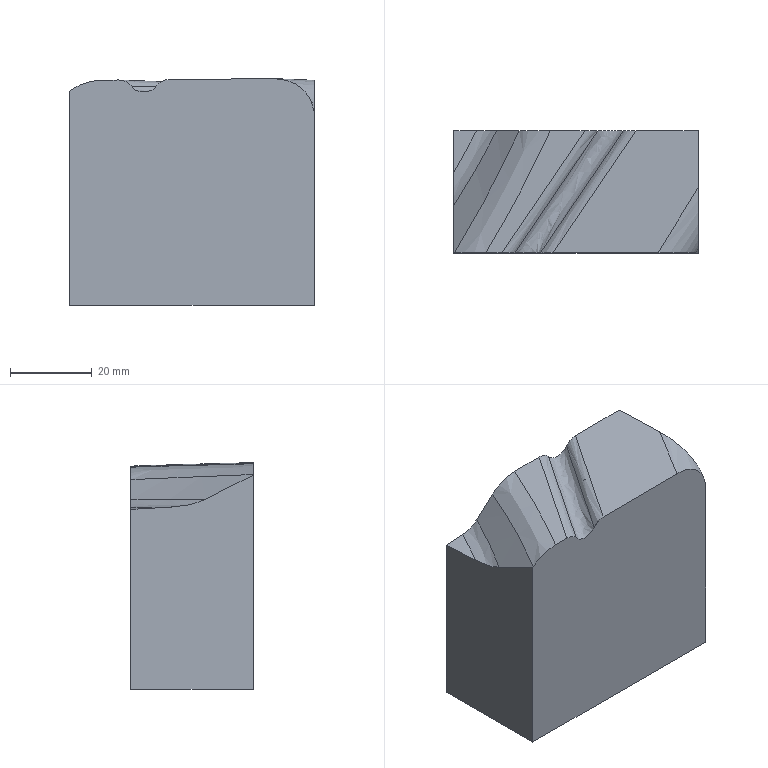Part | NX | features solid 2 | 1 solid | 17 faces | box 60 x 30 x 55.649 mm | volume 96446 mm3 | spline 12 | plane 5
STEP:
#1=CARTESIAN_POINT('',(484.173,-140.,-5.));
#2=VERTEX_POINT('',#1);
#3=CARTESIAN_POINT('',(424.173,-140.,-5.));
#4=VERTEX_POINT('',#3);
#5=CARTESIAN_POINT('',(484.173,-140.,-5.));
#6=DIRECTION('',(1.,0.,0.));
#7=VECTOR('',#6,1000.);
#8=LINE('',#5,#7);
#9=EDGE_CURVE('',#2,#4,#8,.F.);
#10=ORIENTED_EDGE('',*,*,#9,.F.);
#11=CARTESIAN_POINT('',(484.173,-170.,-5.));
#12=VERTEX_POINT('',#11);
#13=CARTESIAN_POINT('',(484.173,-140.,-5.));
#14=DIRECTION('',(0.,1.,0.));
#15=VECTOR('',#14,1000.);
#16=LINE('',#13,#15);
#17=EDGE_CURVE('',#2,#12,#16,.F.);
#18=ORIENTED_EDGE('',*,*,#17,.T.);
#19=CARTESIAN_POINT('',(424.173,-170.,-5.));
#20=VERTEX_POINT('',#19);
#21=CARTESIAN_POINT('',(374.173,-170.,-5.));
#22=DIRECTION('',(-1.,0.,0.));
#23=VECTOR('',#22,1000.);
#24=LINE('',#21,#23);
#25=EDGE_CURVE('',#12,#20,#24,.T.);
#26=ORIENTED_EDGE('',*,*,#25,.T.);
#27=CARTESIAN_POINT('',(424.173,-140.,-5.));
#28=DIRECTION('',(0.,1.,0.));
#29=VECTOR('',#28,1000.);
#30=LINE('',#27,#29);
#31=EDGE_CURVE('',#4,#20,#30,.F.);
#32=ORIENTED_EDGE('',*,*,#31,.F.);
#33=EDGE_LOOP('',(#10,#18,#26,#32));
#34=FACE_BOUND('',#33,.T.);
#35=CARTESIAN_POINT('',(374.173,-140.,-5.));
#36=DIRECTION('',(0.,0.,-1.));
#37=DIRECTION('',(-1.,0.,0.));
#38=AXIS2_PLACEMENT_3D('',#35,#36,#37);
#39=PLANE('',#38);
#40=ADVANCED_FACE('',(#34),#39,.T.);
#41=CARTESIAN_POINT('',(424.173,-170.,47.58));
#42=VERTEX_POINT('',#41);
#43=CARTESIAN_POINT('',(424.173,-170.,115.));
#44=DIRECTION('',(0.,0.,1.));
#45=VECTOR('',#44,1000.);
#46=LINE('',#43,#45);
#47=EDGE_CURVE('',#42,#20,#46,.F.);
#48=ORIENTED_EDGE('',*,*,#47,.T.);
#49=ORIENTED_EDGE('',*,*,#25,.F.);
#50=CARTESIAN_POINT('',(484.173,-170.,42.661));
#51=VERTEX_POINT('',#50);
#52=CARTESIAN_POINT('',(484.173,-170.,115.));
#53=DIRECTION('',(0.,0.,-1.));
#54=VECTOR('',#53,1000.);
#55=LINE('',#52,#54);
#56=EDGE_CURVE('',#51,#12,#55,.T.);
#57=ORIENTED_EDGE('',*,*,#56,.F.);
#58=CARTESIAN_POINT('',(483.509,-170.,44.696));
#59=VERTEX_POINT('',#58);
#60=CARTESIAN_POINT('',(483.509,-170.,44.695));
#61=CARTESIAN_POINT('',(483.73,-170.,44.017));
#62=CARTESIAN_POINT('',(483.952,-170.,43.339));
#63=CARTESIAN_POINT('',(484.173,-170.,42.661));
#64=B_SPLINE_CURVE_WITH_KNOTS('',3,(#60,#61,#62,#63),.UNSPECIFIED.,.F.,.F.,(4,4),(0.017,0.01914),.UNSPECIFIED.);
#65=EDGE_CURVE('',#59,#51,#64,.T.);
#66=ORIENTED_EDGE('',*,*,#65,.F.);
#67=CARTESIAN_POINT('',(474.524,-170.,50.648));
#68=VERTEX_POINT('',#67);
#69=CARTESIAN_POINT('',(474.524,-170.,50.648));
#70=CARTESIAN_POINT('',(476.454,-170.,50.62));
#71=CARTESIAN_POINT('',(480.234,-170.,49.577));
#72=CARTESIAN_POINT('',(482.907,-170.,46.539));
#73=CARTESIAN_POINT('',(483.508,-170.,44.696));
#74=B_SPLINE_CURVE_WITH_KNOTS('',3,(#69,#70,#71,#72,#73),.UNSPECIFIED.,.F.,.F.,(4,1,4),(0.,0.005687,0.01137),.UNSPECIFIED.);
#75=EDGE_CURVE('',#68,#59,#74,.T.);
#76=ORIENTED_EDGE('',*,*,#75,.F.);
#77=CARTESIAN_POINT('',(474.268,-170.,50.649));
#78=VERTEX_POINT('',#77);
#79=CARTESIAN_POINT('',(474.268,-170.,50.649));
#80=CARTESIAN_POINT('',(474.354,-170.,50.649));
#81=CARTESIAN_POINT('',(474.439,-170.,50.649));
#82=CARTESIAN_POINT('',(474.524,-170.,50.648));
#83=B_SPLINE_CURVE_WITH_KNOTS('',3,(#79,#80,#81,#82),.UNSPECIFIED.,.F.,.F.,(4,4),(0.,0.0002558),.UNSPECIFIED.);
#84=EDGE_CURVE('',#78,#68,#83,.T.);
#85=ORIENTED_EDGE('',*,*,#84,.F.);
#86=CARTESIAN_POINT('',(448.584,-170.,50.424));
#87=VERTEX_POINT('',#86);
#88=CARTESIAN_POINT('',(484.734,-170.,50.74));
#89=DIRECTION('',(-1.,0.,-0.008731));
#90=VECTOR('',#89,1000.);
#91=LINE('',#88,#90);
#92=EDGE_CURVE('',#87,#78,#91,.F.);
#93=ORIENTED_EDGE('',*,*,#92,.F.);
#94=CARTESIAN_POINT('',(445.49,-170.,48.897));
#95=VERTEX_POINT('',#94);
#96=CARTESIAN_POINT('',(445.49,-170.,48.897));
#97=CARTESIAN_POINT('',(446.157,-170.,49.903));
#98=CARTESIAN_POINT('',(447.38,-170.,50.414));
#99=CARTESIAN_POINT('',(448.584,-170.,50.424));
#100=B_SPLINE_CURVE_WITH_KNOTS('',3,(#96,#97,#98,#99),.UNSPECIFIED.,.F.,.F.,(4,4),(0.0000186,0.003585),.UNSPECIFIED.);
#101=EDGE_CURVE('',#95,#87,#100,.T.);
#102=ORIENTED_EDGE('',*,*,#101,.F.);
#103=CARTESIAN_POINT('',(439.21,-170.,48.842));
#104=VERTEX_POINT('',#103);
#105=CARTESIAN_POINT('',(439.21,-170.,48.842));
#106=CARTESIAN_POINT('',(440.629,-170.,46.903));
#107=CARTESIAN_POINT('',(444.144,-170.,46.868));
#108=CARTESIAN_POINT('',(445.49,-170.,48.896));
#109=B_SPLINE_CURVE_WITH_KNOTS('',3,(#105,#106,#107,#108),.UNSPECIFIED.,.F.,.F.,(4,4),(0.0007156,0.007904),.UNSPECIFIED.);
#110=EDGE_CURVE('',#104,#95,#109,.T.);
#111=ORIENTED_EDGE('',*,*,#110,.F.);
#112=CARTESIAN_POINT('',(436.025,-170.,50.315));
#113=VERTEX_POINT('',#112);
#114=CARTESIAN_POINT('',(436.025,-170.,50.315));
#115=CARTESIAN_POINT('',(437.248,-170.,50.325));
#116=CARTESIAN_POINT('',(438.485,-170.,49.832));
#117=CARTESIAN_POINT('',(439.21,-170.,48.842));
#118=B_SPLINE_CURVE_WITH_KNOTS('',3,(#114,#115,#116,#117),.UNSPECIFIED.,.F.,.F.,(4,4),(0.00002144,0.003637),.UNSPECIFIED.);
#119=EDGE_CURVE('',#113,#104,#118,.T.);
#120=ORIENTED_EDGE('',*,*,#119,.F.);
#121=CARTESIAN_POINT('',(432.047,-170.,50.28));
#122=VERTEX_POINT('',#121);
#123=CARTESIAN_POINT('',(484.734,-170.,50.74));
#124=DIRECTION('',(-1.,0.,-0.008731));
#125=VECTOR('',#124,1000.);
#126=LINE('',#123,#125);
#127=EDGE_CURVE('',#122,#113,#126,.F.);
#128=ORIENTED_EDGE('',*,*,#127,.F.);
#129=CARTESIAN_POINT('',(424.373,-170.,47.733));
#130=VERTEX_POINT('',#129);
#131=CARTESIAN_POINT('',(424.373,-170.,47.733));
#132=CARTESIAN_POINT('',(426.555,-170.,49.407));
#133=CARTESIAN_POINT('',(429.292,-170.,50.256));
#134=CARTESIAN_POINT('',(432.047,-170.,50.28));
#135=B_SPLINE_CURVE_WITH_KNOTS('',3,(#131,#132,#133,#134),.UNSPECIFIED.,.F.,.F.,(4,4),(-0.0009759,0.007265),.UNSPECIFIED.);
#136=EDGE_CURVE('',#130,#122,#135,.T.);
#137=ORIENTED_EDGE('',*,*,#136,.F.);
#138=CARTESIAN_POINT('',(424.173,-170.,47.58));
#139=CARTESIAN_POINT('',(424.24,-170.,47.631));
#140=CARTESIAN_POINT('',(424.306,-170.,47.682));
#141=CARTESIAN_POINT('',(424.373,-170.,47.733));
#142=B_SPLINE_CURVE_WITH_KNOTS('',3,(#138,#139,#140,#141),.UNSPECIFIED.,.F.,.F.,(4,4),(0.,0.0002516),.UNSPECIFIED.);
#143=EDGE_CURVE('',#42,#130,#142,.T.);
#144=ORIENTED_EDGE('',*,*,#143,.F.);
#145=EDGE_LOOP('',(#48,#49,#57,#66,#76,#85,#93,#102,#111,#120,#128,#137,#144));
#146=FACE_BOUND('',#145,.T.);
#147=CARTESIAN_POINT('',(484.173,-170.,115.));
#148=DIRECTION('',(0.,-1.,0.));
#149=DIRECTION('',(0.,0.,-1.));
#150=AXIS2_PLACEMENT_3D('',#147,#148,#149);
#151=PLANE('',#150);
#152=ADVANCED_FACE('',(#146),#151,.T.);
#153=CARTESIAN_POINT('',(434.724,-140.,41.512));
#154=VERTEX_POINT('',#153);
#155=CARTESIAN_POINT('',(429.796,-140.,39.524));
#156=VERTEX_POINT('',#155);
#157=CARTESIAN_POINT('',(434.724,-140.,41.512));
#158=CARTESIAN_POINT('',(433.368,-140.,40.305));
#159=CARTESIAN_POINT('',(431.606,-140.,39.634));
#160=CARTESIAN_POINT('',(429.796,-140.,39.524));
#161=B_SPLINE_CURVE_WITH_KNOTS('',3,(#157,#158,#159,#160),.UNSPECIFIED.,.F.,.F.,(4,4),(0.,0.005426),.UNSPECIFIED.);
#162=EDGE_CURVE('',#154,#156,#161,.T.);
#163=ORIENTED_EDGE('',*,*,#162,.F.);
#164=CARTESIAN_POINT('',(440.182,-140.,46.484));
#165=VERTEX_POINT('',#164);
#166=CARTESIAN_POINT('',(440.182,-140.,46.484));
#167=CARTESIAN_POINT('',(438.381,-140.,44.806));
#168=CARTESIAN_POINT('',(436.562,-140.,43.148));
#169=CARTESIAN_POINT('',(434.724,-140.,41.512));
#170=B_SPLINE_CURVE_WITH_KNOTS('',3,(#166,#167,#168,#169),.UNSPECIFIED.,.F.,.F.,(4,4),(0.003756,0.01114),.UNSPECIFIED.);
#171=EDGE_CURVE('',#165,#154,#170,.T.);
#172=ORIENTED_EDGE('',*,*,#171,.F.);
#173=CARTESIAN_POINT('',(447.906,-140.,49.476));
#174=VERTEX_POINT('',#173);
#175=CARTESIAN_POINT('',(447.906,-140.,49.476));
#176=CARTESIAN_POINT('',(445.063,-140.,49.451));
#177=CARTESIAN_POINT('',(442.263,-140.,48.423));
#178=CARTESIAN_POINT('',(440.182,-140.,46.484));
#179=B_SPLINE_CURVE_WITH_KNOTS('',3,(#175,#176,#177,#178),.UNSPECIFIED.,.F.,.F.,(4,4),(0.,0.0084),.UNSPECIFIED.);
#180=EDGE_CURVE('',#174,#165,#179,.T.);
#181=ORIENTED_EDGE('',*,*,#180,.F.);
#182=CARTESIAN_POINT('',(456.404,-140.,49.55));
#183=VERTEX_POINT('',#182);
#184=CARTESIAN_POINT('',(484.742,-140.,49.797));
#185=DIRECTION('',(-1.,0.,-0.008731));
#186=VECTOR('',#185,1000.);
#187=LINE('',#184,#186);
#188=EDGE_CURVE('',#183,#174,#187,.T.);
#189=ORIENTED_EDGE('',*,*,#188,.F.);
#190=CARTESIAN_POINT('',(459.589,-140.,48.077));
#191=VERTEX_POINT('',#190);
#192=CARTESIAN_POINT('',(459.589,-140.,48.077));
#193=CARTESIAN_POINT('',(458.865,-140.,49.066));
#194=CARTESIAN_POINT('',(457.625,-140.,49.561));
#195=CARTESIAN_POINT('',(456.404,-140.,49.55));
#196=B_SPLINE_CURVE_WITH_KNOTS('',3,(#192,#193,#194,#195),.UNSPECIFIED.,.F.,.F.,(4,4),(0.00001889,0.00364),.UNSPECIFIED.);
#197=EDGE_CURVE('',#191,#183,#196,.T.);
#198=ORIENTED_EDGE('',*,*,#197,.F.);
#199=CARTESIAN_POINT('',(465.869,-140.,48.132));
#200=VERTEX_POINT('',#199);
#201=CARTESIAN_POINT('',(465.869,-140.,48.132));
#202=CARTESIAN_POINT('',(465.195,-140.,47.116));
#203=CARTESIAN_POINT('',(462.737,-140.,46.1));
#204=CARTESIAN_POINT('',(460.304,-140.,47.1));
#205=CARTESIAN_POINT('',(459.589,-140.,48.077));
#206=B_SPLINE_CURVE_WITH_KNOTS('',3,(#201,#202,#203,#204,#205),.UNSPECIFIED.,.F.,.F.,(4,1,4),(0.,0.003598,0.007195),.UNSPECIFIED.);
#207=EDGE_CURVE('',#200,#191,#206,.T.);
#208=ORIENTED_EDGE('',*,*,#207,.F.);
#209=CARTESIAN_POINT('',(468.963,-140.,49.66));
#210=VERTEX_POINT('',#209);
#211=CARTESIAN_POINT('',(468.963,-140.,49.66));
#212=CARTESIAN_POINT('',(467.759,-140.,49.649));
#213=CARTESIAN_POINT('',(466.537,-140.,49.139));
#214=CARTESIAN_POINT('',(465.868,-140.,48.132));
#215=B_SPLINE_CURVE_WITH_KNOTS('',3,(#211,#212,#213,#214),.UNSPECIFIED.,.F.,.F.,(4,4),(0.00002143,0.003581),.UNSPECIFIED.);
#216=EDGE_CURVE('',#210,#200,#215,.T.);
#217=ORIENTED_EDGE('',*,*,#216,.F.);
#218=CARTESIAN_POINT('',(484.173,-140.,49.792));
#219=VERTEX_POINT('',#218);
#220=CARTESIAN_POINT('',(484.742,-140.,49.797));
#221=DIRECTION('',(-1.,0.,-0.008731));
#222=VECTOR('',#221,1000.);
#223=LINE('',#220,#222);
#224=EDGE_CURVE('',#219,#210,#223,.T.);
#225=ORIENTED_EDGE('',*,*,#224,.F.);
#226=CARTESIAN_POINT('',(484.173,-140.,115.));
#227=DIRECTION('',(0.,0.,-1.));
#228=VECTOR('',#227,1000.);
#229=LINE('',#226,#228);
#230=EDGE_CURVE('',#219,#2,#229,.T.);
#231=ORIENTED_EDGE('',*,*,#230,.T.);
#232=ORIENTED_EDGE('',*,*,#9,.T.);
#233=CARTESIAN_POINT('',(424.173,-140.,39.179));
#234=VERTEX_POINT('',#233);
#235=CARTESIAN_POINT('',(424.173,-140.,115.));
#236=DIRECTION('',(0.,0.,-1.));
#237=VECTOR('',#236,1000.);
#238=LINE('',#235,#237);
#239=EDGE_CURVE('',#234,#4,#238,.T.);
#240=ORIENTED_EDGE('',*,*,#239,.F.);
#241=CARTESIAN_POINT('',(429.796,-140.,39.524));
#242=CARTESIAN_POINT('',(427.922,-140.,39.409));
#243=CARTESIAN_POINT('',(426.047,-140.,39.294));
#244=CARTESIAN_POINT('',(424.173,-140.,39.179));
#245=B_SPLINE_CURVE_WITH_KNOTS('',3,(#241,#242,#243,#244),.UNSPECIFIED.,.F.,.F.,(4,4),(0.01255,0.01818),.UNSPECIFIED.);
#246=EDGE_CURVE('',#156,#234,#245,.T.);
#247=ORIENTED_EDGE('',*,*,#246,.F.);
#248=EDGE_LOOP('',(#163,#172,#181,#189,#198,#208,#217,#225,#231,#232,#240,#247));
#249=FACE_BOUND('',#248,.T.);
#250=CARTESIAN_POINT('',(484.173,-140.,115.));
#251=DIRECTION('',(0.,-1.,0.));
#252=DIRECTION('',(0.,0.,-1.));
#253=AXIS2_PLACEMENT_3D('',#250,#251,#252);
#254=PLANE('',#253);
#255=ADVANCED_FACE('',(#249),#254,.F.);
#256=CARTESIAN_POINT('',(484.173,-168.915,44.667));
#257=VERTEX_POINT('',#256);
#258=CARTESIAN_POINT('',(484.173,-153.965,50.231));
#259=VERTEX_POINT('',#258);
#260=CARTESIAN_POINT('',(484.173,-168.914,44.669));
#261=CARTESIAN_POINT('',(484.173,-168.241,45.912));
#262=CARTESIAN_POINT('',(484.173,-166.076,47.753));
#263=CARTESIAN_POINT('',(484.173,-162.195,49.352));
#264=CARTESIAN_POINT('',(484.173,-158.143,50.156));
#265=CARTESIAN_POINT('',(484.173,-155.352,50.275));
#266=CARTESIAN_POINT('',(484.173,-153.962,50.231));
#267=B_SPLINE_CURVE_WITH_KNOTS('',3,(#260,#261,#262,#263,#264,#265,#266),.UNSPECIFIED.,.F.,.F.,(4,1,1,1,4),(0.,0.004145,0.008291,0.01244,0.01658),.UNSPECIFIED.);
#268=EDGE_CURVE('',#257,#259,#267,.T.);
#269=ORIENTED_EDGE('',*,*,#268,.F.);
#270=CARTESIAN_POINT('',(484.173,-170.,42.661));
#271=CARTESIAN_POINT('',(484.173,-169.638,43.329));
#272=CARTESIAN_POINT('',(484.173,-169.277,43.998));
#273=CARTESIAN_POINT('',(484.173,-168.915,44.666));
#274=B_SPLINE_CURVE_WITH_KNOTS('',3,(#270,#271,#272,#273),.UNSPECIFIED.,.F.,.F.,(4,4),(0.,0.00228),.UNSPECIFIED.);
#275=EDGE_CURVE('',#51,#257,#274,.T.);
#276=ORIENTED_EDGE('',*,*,#275,.F.);
#277=ORIENTED_EDGE('',*,*,#56,.T.);
#278=ORIENTED_EDGE('',*,*,#17,.F.);
#279=ORIENTED_EDGE('',*,*,#230,.F.);
#280=CARTESIAN_POINT('',(484.173,-142.047,49.857));
#281=DIRECTION('',(0.,0.9995,-0.03141));
#282=VECTOR('',#281,1000.);
#283=LINE('',#280,#282);
#284=EDGE_CURVE('',#259,#219,#283,.T.);
#285=ORIENTED_EDGE('',*,*,#284,.F.);
#286=EDGE_LOOP('',(#269,#276,#277,#278,#279,#285));
#287=FACE_BOUND('',#286,.T.);
#288=CARTESIAN_POINT('',(484.173,-140.,115.));
#289=DIRECTION('',(-1.,0.,0.));
#290=DIRECTION('',(0.,0.,-1.));
#291=AXIS2_PLACEMENT_3D('',#288,#289,#290);
#292=PLANE('',#291);
#293=ADVANCED_FACE('',(#287),#292,.F.);
#294=ORIENTED_EDGE('',*,*,#47,.F.);
#295=CARTESIAN_POINT('',(424.173,-158.353,41.69));
#296=VERTEX_POINT('',#295);
#297=CARTESIAN_POINT('',(424.173,-170.,47.58));
#298=CARTESIAN_POINT('',(424.173,-166.121,45.609));
#299=CARTESIAN_POINT('',(424.173,-162.239,43.646));
#300=CARTESIAN_POINT('',(424.173,-158.353,41.69));
#301=B_SPLINE_CURVE_WITH_KNOTS('',3,(#297,#298,#299,#300),.UNSPECIFIED.,.F.,.F.,(4,4),(0.0003673,0.01342),.UNSPECIFIED.);
#302=EDGE_CURVE('',#42,#296,#301,.T.);
#303=ORIENTED_EDGE('',*,*,#302,.T.);
#304=CARTESIAN_POINT('',(424.173,-150.298,39.769));
#305=VERTEX_POINT('',#304);
#306=CARTESIAN_POINT('',(424.173,-150.298,39.769));
#307=CARTESIAN_POINT('',(424.173,-153.074,39.92));
#308=CARTESIAN_POINT('',(424.173,-155.868,40.438));
#309=CARTESIAN_POINT('',(424.173,-158.354,41.69));
#310=B_SPLINE_CURVE_WITH_KNOTS('',3,(#306,#307,#308,#309),.UNSPECIFIED.,.F.,.F.,(4,4),(0.03155,0.03989),.UNSPECIFIED.);
#311=EDGE_CURVE('',#296,#305,#310,.F.);
#312=ORIENTED_EDGE('',*,*,#311,.T.);
#313=CARTESIAN_POINT('',(424.173,-150.298,39.769));
#314=CARTESIAN_POINT('',(424.173,-146.865,39.582));
#315=CARTESIAN_POINT('',(424.173,-143.432,39.385));
#316=CARTESIAN_POINT('',(424.173,-140.,39.179));
#317=B_SPLINE_CURVE_WITH_KNOTS('',3,(#313,#314,#315,#316),.UNSPECIFIED.,.F.,.F.,(4,4),(0.0757,0.08601),.UNSPECIFIED.);
#318=EDGE_CURVE('',#305,#234,#317,.T.);
#319=ORIENTED_EDGE('',*,*,#318,.T.);
#320=ORIENTED_EDGE('',*,*,#239,.T.);
#321=ORIENTED_EDGE('',*,*,#31,.T.);
#322=EDGE_LOOP('',(#294,#303,#312,#319,#320,#321));
#323=FACE_BOUND('',#322,.T.);
#324=CARTESIAN_POINT('',(424.173,-140.,115.));
#325=DIRECTION('',(-1.,0.,0.));
#326=DIRECTION('',(0.,0.,-1.));
#327=AXIS2_PLACEMENT_3D('',#324,#325,#326);
#328=PLANE('',#327);
#329=ADVANCED_FACE('',(#323),#328,.T.);
#330=CARTESIAN_POINT('',(484.173,-168.914,44.669));
#331=CARTESIAN_POINT('',(483.951,-169.276,44.678));
#332=CARTESIAN_POINT('',(483.73,-169.638,44.687));
#333=CARTESIAN_POINT('',(483.508,-170.,44.696));
#334=B_SPLINE_CURVE_WITH_KNOTS('',3,(#330,#331,#332,#333),.UNSPECIFIED.,.F.,.F.,(4,4),(0.9687,0.9753),.UNSPECIFIED.);
#335=EDGE_CURVE('',#59,#257,#334,.F.);
#336=ORIENTED_EDGE('',*,*,#335,.T.);
#337=ORIENTED_EDGE('',*,*,#268,.T.);
#338=CARTESIAN_POINT('',(474.337,-169.887,50.646));
#339=VERTEX_POINT('',#338);
#340=CARTESIAN_POINT('',(474.337,-169.887,50.646));
#341=CARTESIAN_POINT('',(477.558,-164.566,50.507));
#342=CARTESIAN_POINT('',(480.838,-159.247,50.368));
#343=CARTESIAN_POINT('',(484.17,-153.966,50.231));
#344=B_SPLINE_CURVE_WITH_KNOTS('',3,(#340,#341,#342,#343),.UNSPECIFIED.,.F.,.F.,(4,4),(0.,0.09571),.UNSPECIFIED.);
#345=EDGE_CURVE('',#339,#259,#344,.T.);
#346=ORIENTED_EDGE('',*,*,#345,.F.);
#347=CARTESIAN_POINT('',(481.023,-174.087,44.801));
#348=CARTESIAN_POINT('',(480.792,-173.92,45.819));
#349=CARTESIAN_POINT('',(480.416,-173.667,46.791));
#350=CARTESIAN_POINT('',(479.903,-173.334,47.678));
#351=CARTESIAN_POINT('',(478.645,-172.532,49.218));
#352=CARTESIAN_POINT('',(477.023,-171.525,50.196));
#353=CARTESIAN_POINT('',(476.148,-170.987,50.521));
#354=CARTESIAN_POINT('',(475.242,-170.434,50.671));
#355=CARTESIAN_POINT('',(474.337,-169.887,50.646));
#356=B_SPLINE_CURVE_WITH_KNOTS('',5,(#347,#348,#349,#350,#351,#352,#353,#354,#355),.UNSPECIFIED.,.F.,.F.,(6,3,6),(0.,0.5,1.),.UNSPECIFIED.);
#357=EDGE_CURVE('',#339,#68,#356,.F.);
#358=ORIENTED_EDGE('',*,*,#357,.T.);
#359=ORIENTED_EDGE('',*,*,#75,.T.);
#360=EDGE_LOOP('',(#336,#337,#346,#358,#359));
#361=FACE_BOUND('',#360,.T.);
#362=CARTESIAN_POINT('',(481.023,-174.087,44.801));
#363=CARTESIAN_POINT('',(480.792,-173.92,45.819));
#364=CARTESIAN_POINT('',(480.416,-173.667,46.791));
#365=CARTESIAN_POINT('',(479.903,-173.334,47.678));
#366=CARTESIAN_POINT('',(478.645,-172.532,49.218));
#367=CARTESIAN_POINT('',(477.023,-171.525,50.196));
#368=CARTESIAN_POINT('',(476.148,-170.987,50.521));
#369=CARTESIAN_POINT('',(475.242,-170.434,50.671));
#370=CARTESIAN_POINT('',(474.337,-169.887,50.646));
#371=CARTESIAN_POINT('',(481.288,-173.65,44.789));
#372=CARTESIAN_POINT('',(481.057,-173.483,45.808));
#373=CARTESIAN_POINT('',(480.681,-173.229,46.78));
#374=CARTESIAN_POINT('',(480.168,-172.896,47.667));
#375=CARTESIAN_POINT('',(478.91,-172.093,49.207));
#376=CARTESIAN_POINT('',(477.289,-171.086,50.184));
#377=CARTESIAN_POINT('',(476.414,-170.547,50.51));
#378=CARTESIAN_POINT('',(475.508,-169.994,50.659));
#379=CARTESIAN_POINT('',(474.603,-169.446,50.634));
#380=CARTESIAN_POINT('',(481.553,-173.213,44.778));
#381=CARTESIAN_POINT('',(481.321,-173.046,45.797));
#382=CARTESIAN_POINT('',(480.945,-172.792,46.768));
#383=CARTESIAN_POINT('',(480.433,-172.458,47.656));
#384=CARTESIAN_POINT('',(479.175,-171.655,49.195));
#385=CARTESIAN_POINT('',(477.555,-170.647,50.173));
#386=CARTESIAN_POINT('',(476.681,-170.108,50.498));
#387=CARTESIAN_POINT('',(475.775,-169.554,50.648));
#388=CARTESIAN_POINT('',(474.87,-169.006,50.623));
#389=CARTESIAN_POINT('',(481.816,-172.778,44.767));
#390=CARTESIAN_POINT('',(481.585,-172.611,45.786));
#391=CARTESIAN_POINT('',(481.209,-172.357,46.757));
#392=CARTESIAN_POINT('',(480.697,-172.023,47.644));
#393=CARTESIAN_POINT('',(479.439,-171.22,49.184));
#394=CARTESIAN_POINT('',(477.82,-170.211,50.162));
#395=CARTESIAN_POINT('',(476.945,-169.671,50.487));
#396=CARTESIAN_POINT('',(476.04,-169.118,50.636));
#397=CARTESIAN_POINT('',(475.135,-168.569,50.611));
#398=CARTESIAN_POINT('',(483.192,-170.514,44.709));
#399=CARTESIAN_POINT('',(482.961,-170.346,45.728));
#400=CARTESIAN_POINT('',(482.585,-170.092,46.699));
#401=CARTESIAN_POINT('',(482.074,-169.756,47.586));
#402=CARTESIAN_POINT('',(480.818,-168.95,49.125));
#403=CARTESIAN_POINT('',(479.201,-167.937,50.102));
#404=CARTESIAN_POINT('',(478.328,-167.396,50.427));
#405=CARTESIAN_POINT('',(477.423,-166.84,50.577));
#406=CARTESIAN_POINT('',(476.521,-166.289,50.552));
#407=CARTESIAN_POINT('',(484.575,-168.252,44.652));
#408=CARTESIAN_POINT('',(484.344,-168.084,45.67));
#409=CARTESIAN_POINT('',(483.969,-167.828,46.641));
#410=CARTESIAN_POINT('',(483.458,-167.492,47.528));
#411=CARTESIAN_POINT('',(482.204,-166.682,49.066));
#412=CARTESIAN_POINT('',(480.59,-165.665,50.043));
#413=CARTESIAN_POINT('',(479.718,-165.122,50.368));
#414=CARTESIAN_POINT('',(478.816,-164.564,50.518));
#415=CARTESIAN_POINT('',(477.914,-164.011,50.492));
#416=CARTESIAN_POINT('',(485.697,-166.429,44.606));
#417=CARTESIAN_POINT('',(485.466,-166.26,45.624));
#418=CARTESIAN_POINT('',(485.091,-166.003,46.595));
#419=CARTESIAN_POINT('',(484.581,-165.666,47.481));
#420=CARTESIAN_POINT('',(483.329,-164.853,49.019));
#421=CARTESIAN_POINT('',(481.717,-163.833,49.996));
#422=CARTESIAN_POINT('',(480.847,-163.287,50.32));
#423=CARTESIAN_POINT('',(479.945,-162.727,50.47));
#424=CARTESIAN_POINT('',(479.046,-162.173,50.444));
#425=CARTESIAN_POINT('',(487.396,-163.683,44.537));
#426=CARTESIAN_POINT('',(487.165,-163.514,45.554));
#427=CARTESIAN_POINT('',(486.792,-163.256,46.525));
#428=CARTESIAN_POINT('',(486.283,-162.917,47.411));
#429=CARTESIAN_POINT('',(485.033,-162.1,48.948));
#430=CARTESIAN_POINT('',(483.425,-161.074,49.924));
#431=CARTESIAN_POINT('',(482.556,-160.526,50.249));
#432=CARTESIAN_POINT('',(481.657,-159.963,50.398));
#433=CARTESIAN_POINT('',(480.759,-159.406,50.372));
#434=CARTESIAN_POINT('',(489.108,-160.945,44.467));
#435=CARTESIAN_POINT('',(488.877,-160.774,45.485));
#436=CARTESIAN_POINT('',(488.504,-160.515,46.455));
#437=CARTESIAN_POINT('',(487.996,-160.174,47.341));
#438=CARTESIAN_POINT('',(486.749,-159.353,48.877));
#439=CARTESIAN_POINT('',(485.144,-158.322,49.853));
#440=CARTESIAN_POINT('',(484.278,-157.772,50.177));
#441=CARTESIAN_POINT('',(483.381,-157.206,50.326));
#442=CARTESIAN_POINT('',(482.485,-156.645,50.301));
#443=CARTESIAN_POINT('',(489.684,-160.025,44.444));
#444=CARTESIAN_POINT('',(489.454,-159.854,45.461));
#445=CARTESIAN_POINT('',(489.081,-159.594,46.431));
#446=CARTESIAN_POINT('',(488.574,-159.253,47.317));
#447=CARTESIAN_POINT('',(487.328,-158.43,48.854));
#448=CARTESIAN_POINT('',(485.724,-157.398,49.829));
#449=CARTESIAN_POINT('',(484.858,-156.846,50.153));
#450=CARTESIAN_POINT('',(483.962,-156.279,50.302));
#451=CARTESIAN_POINT('',(483.067,-155.718,50.277));
#452=CARTESIAN_POINT('',(490.262,-159.106,44.421));
#453=CARTESIAN_POINT('',(490.032,-158.934,45.438));
#454=CARTESIAN_POINT('',(489.659,-158.675,46.408));
#455=CARTESIAN_POINT('',(489.152,-158.332,47.294));
#456=CARTESIAN_POINT('',(487.907,-157.509,48.83));
#457=CARTESIAN_POINT('',(486.304,-156.475,49.805));
#458=CARTESIAN_POINT('',(485.44,-155.922,50.129));
#459=CARTESIAN_POINT('',(484.544,-155.354,50.278));
#460=CARTESIAN_POINT('',(483.649,-154.792,50.253));
#461=CARTESIAN_POINT('',(490.841,-158.188,44.398));
#462=CARTESIAN_POINT('',(490.611,-158.016,45.415));
#463=CARTESIAN_POINT('',(490.239,-157.756,46.384));
#464=CARTESIAN_POINT('',(489.732,-157.413,47.27));
#465=CARTESIAN_POINT('',(488.488,-156.588,48.806));
#466=CARTESIAN_POINT('',(486.886,-155.552,49.781));
#467=CARTESIAN_POINT('',(486.022,-154.999,50.105));
#468=CARTESIAN_POINT('',(485.127,-154.43,50.254));
#469=CARTESIAN_POINT('',(484.233,-153.867,50.229));
#470=B_SPLINE_SURFACE_WITH_KNOTS('',5,5,((#362,#363,#364,#365,#366,#367,#368,#369,#370),(#371,#372,#373,#374,#375,#376,#377,#378,#379),(#380,#381,#382,#383,#384,#385,#386,#387,#388),(#389,#390,#391,#392,#393,#394,#395,#396,#397),(#398,#399,#400,#401,#402,#403,#404,#405,#406),(#407,#408,#409,#410,#411,#412,#413,#414,#415),(#416,#417,#418,#419,#420,#421,#422,#423,#424),(#425,#426,#427,#428,#429,#430,#431,#432,#433),(#434,#435,#436,#437,#438,#439,#440,#441,#442),(#443,#444,#445,#446,#447,#448,#449,#450,#451),(#452,#453,#454,#455,#456,#457,#458,#459,#460),(#461,#462,#463,#464,#465,#466,#467,#468,#469)),.UNSPECIFIED.,.F.,.F.,.F.,(6,3,3,6),(6,3,6),(0.,0.0132,0.06836,0.09631),(0.,0.5,1.),.UNSPECIFIED.);
#471=ADVANCED_FACE('',(#361),#470,.T.);
#472=CARTESIAN_POINT('',(474.268,-170.,50.649));
#473=CARTESIAN_POINT('',(474.291,-169.962,50.648));
#474=CARTESIAN_POINT('',(474.314,-169.925,50.647));
#475=CARTESIAN_POINT('',(474.337,-169.887,50.646));
#476=B_SPLINE_CURVE_WITH_KNOTS('',3,(#472,#473,#474,#475),.UNSPECIFIED.,.F.,.F.,(4,4),(0.9877,1.),.UNSPECIFIED.);
#477=EDGE_CURVE('',#78,#339,#476,.T.);
#478=ORIENTED_EDGE('',*,*,#477,.F.);
#479=ORIENTED_EDGE('',*,*,#84,.T.);
#480=ORIENTED_EDGE('',*,*,#357,.F.);
#481=EDGE_LOOP('',(#478,#479,#480));
#482=FACE_BOUND('',#481,.T.);
#483=CARTESIAN_POINT('',(474.456,-170.115,50.651));
#484=CARTESIAN_POINT('',(474.419,-170.092,50.651));
#485=CARTESIAN_POINT('',(474.381,-170.069,50.651));
#486=CARTESIAN_POINT('',(474.343,-170.046,50.651));
#487=CARTESIAN_POINT('',(474.306,-170.024,50.65));
#488=CARTESIAN_POINT('',(474.268,-170.001,50.649));
#489=CARTESIAN_POINT('',(474.47,-170.092,50.65));
#490=CARTESIAN_POINT('',(474.432,-170.069,50.651));
#491=CARTESIAN_POINT('',(474.395,-170.046,50.65));
#492=CARTESIAN_POINT('',(474.357,-170.024,50.65));
#493=CARTESIAN_POINT('',(474.319,-170.001,50.649));
#494=CARTESIAN_POINT('',(474.282,-169.978,50.648));
#495=CARTESIAN_POINT('',(474.484,-170.069,50.65));
#496=CARTESIAN_POINT('',(474.446,-170.046,50.65));
#497=CARTESIAN_POINT('',(474.409,-170.023,50.65));
#498=CARTESIAN_POINT('',(474.371,-170.001,50.649));
#499=CARTESIAN_POINT('',(474.333,-169.978,50.649));
#500=CARTESIAN_POINT('',(474.295,-169.955,50.648));
#501=CARTESIAN_POINT('',(474.498,-170.046,50.649));
#502=CARTESIAN_POINT('',(474.46,-170.023,50.649));
#503=CARTESIAN_POINT('',(474.422,-170.001,50.649));
#504=CARTESIAN_POINT('',(474.385,-169.978,50.649));
#505=CARTESIAN_POINT('',(474.347,-169.955,50.648));
#506=CARTESIAN_POINT('',(474.309,-169.932,50.647));
#507=CARTESIAN_POINT('',(474.511,-170.023,50.649));
#508=CARTESIAN_POINT('',(474.474,-170.001,50.649));
#509=CARTESIAN_POINT('',(474.436,-169.978,50.649));
#510=CARTESIAN_POINT('',(474.398,-169.955,50.648));
#511=CARTESIAN_POINT('',(474.361,-169.932,50.647));
#512=CARTESIAN_POINT('',(474.323,-169.91,50.646));
#513=CARTESIAN_POINT('',(474.525,-170.001,50.648));
#514=CARTESIAN_POINT('',(474.488,-169.978,50.648));
#515=CARTESIAN_POINT('',(474.45,-169.955,50.648));
#516=CARTESIAN_POINT('',(474.412,-169.932,50.648));
#517=CARTESIAN_POINT('',(474.375,-169.909,50.647));
#518=CARTESIAN_POINT('',(474.337,-169.887,50.646));
#519=B_SPLINE_SURFACE_WITH_KNOTS('',5,5,((#483,#484,#485,#486,#487,#488),(#489,#490,#491,#492,#493,#494),(#495,#496,#497,#498,#499,#500),(#501,#502,#503,#504,#505,#506),(#507,#508,#509,#510,#511,#512),(#513,#514,#515,#516,#517,#518)),.UNSPECIFIED.,.F.,.F.,.F.,(6,6),(6,6),(0.9876,1.),(0.9792,1.),.PIECEWISE_BEZIER_KNOTS.);
#520=ADVANCED_FACE('',(#482),#519,.T.);
#521=ORIENTED_EDGE('',*,*,#65,.T.);
#522=ORIENTED_EDGE('',*,*,#275,.T.);
#523=ORIENTED_EDGE('',*,*,#335,.F.);
#524=EDGE_LOOP('',(#521,#522,#523));
#525=FACE_BOUND('',#524,.T.);
#526=CARTESIAN_POINT('',(484.175,-168.905,44.678));
#527=CARTESIAN_POINT('',(484.539,-169.443,42.568));
#528=CARTESIAN_POINT('',(484.036,-169.118,44.708));
#529=CARTESIAN_POINT('',(484.401,-169.657,42.599));
#530=CARTESIAN_POINT('',(483.897,-169.332,44.739));
#531=CARTESIAN_POINT('',(484.262,-169.87,42.629));
#532=CARTESIAN_POINT('',(483.759,-169.545,44.769));
#533=CARTESIAN_POINT('',(484.123,-170.083,42.659));
#534=CARTESIAN_POINT('',(483.62,-169.759,44.8));
#535=CARTESIAN_POINT('',(483.984,-170.297,42.69));
#536=CARTESIAN_POINT('',(483.481,-169.972,44.83));
#537=CARTESIAN_POINT('',(483.846,-170.51,42.72));
#538=B_SPLINE_SURFACE_WITH_KNOTS('',5,1,((#526,#527),(#528,#529),(#530,#531),(#532,#533),(#534,#535),(#536,#537)),.RULED_SURF.,.F.,.F.,.F.,(6,6),(2,2),(0.9687,0.9754),(0.3431,0.3848),.PIECEWISE_BEZIER_KNOTS.);
#539=ADVANCED_FACE('',(#525),#538,.T.);
#540=ORIENTED_EDGE('',*,*,#302,.F.);
#541=ORIENTED_EDGE('',*,*,#143,.T.);
#542=CARTESIAN_POINT('',(424.373,-170.,47.733));
#543=CARTESIAN_POINT('',(429.952,-160.832,47.36));
#544=CARTESIAN_POINT('',(435.25,-150.825,46.944));
#545=CARTESIAN_POINT('',(440.182,-140.,46.484));
#546=B_SPLINE_CURVE_WITH_KNOTS('',3,(#542,#543,#544,#545),.UNSPECIFIED.,.F.,.F.,(4,4),(0.2507,0.9196),.UNSPECIFIED.);
#547=EDGE_CURVE('',#130,#165,#546,.T.);
#548=ORIENTED_EDGE('',*,*,#547,.T.);
#549=ORIENTED_EDGE('',*,*,#171,.T.);
#550=CARTESIAN_POINT('',(434.724,-140.,41.512));
#551=CARTESIAN_POINT('',(433.047,-143.277,41.583));
#552=CARTESIAN_POINT('',(430.496,-147.982,41.66));
#553=CARTESIAN_POINT('',(427.425,-153.172,41.694));
#554=CARTESIAN_POINT('',(425.695,-155.976,41.698));
#555=CARTESIAN_POINT('',(424.667,-157.591,41.694));
#556=CARTESIAN_POINT('',(424.173,-158.353,41.69));
#557=B_SPLINE_CURVE_WITH_KNOTS('',3,(#550,#551,#552,#553,#554,#555,#556),.UNSPECIFIED.,.F.,.F.,(4,1,1,1,4),(0.1949,0.3725,0.4613,0.5057,0.5501),.UNSPECIFIED.);
#558=EDGE_CURVE('',#154,#296,#557,.T.);
#559=ORIENTED_EDGE('',*,*,#558,.T.);
#560=EDGE_LOOP('',(#540,#541,#548,#549,#559));
#561=FACE_BOUND('',#560,.T.);
#562=CARTESIAN_POINT('',(439.499,-136.687,44.301));
#563=CARTESIAN_POINT('',(444.63,-157.481,58.795));
#564=CARTESIAN_POINT('',(432.956,-141.116,40.264));
#565=CARTESIAN_POINT('',(438.087,-161.909,54.758));
#566=CARTESIAN_POINT('',(426.108,-145.393,36.553));
#567=CARTESIAN_POINT('',(431.239,-166.186,51.047));
#568=CARTESIAN_POINT('',(418.97,-149.504,33.181));
#569=CARTESIAN_POINT('',(424.101,-170.297,47.676));
#570=(BOUNDED_SURFACE()B_SPLINE_SURFACE(3,1,((#562,#563),(#564,#565),(#566,#567),(#568,#569)),.CYLINDRICAL_SURF.,.F.,.F.,.F.)B_SPLINE_SURFACE_WITH_KNOTS((4,4),(2,2),(0.02535,0.2468),(0.1052,0.4262),.PIECEWISE_BEZIER_KNOTS.)GEOMETRIC_REPRESENTATION_ITEM()RATIONAL_B_SPLINE_SURFACE(((0.9986,0.9986),(0.9945,0.9945),(0.9914,0.9914),(0.9892,0.9892)))REPRESENTATION_ITEM('')SURFACE());
#571=ADVANCED_FACE('',(#561),#570,.T.);
#572=ORIENTED_EDGE('',*,*,#547,.F.);
#573=ORIENTED_EDGE('',*,*,#136,.T.);
#574=CARTESIAN_POINT('',(447.906,-140.,49.476));
#575=CARTESIAN_POINT('',(443.18,-150.275,49.757));
#576=CARTESIAN_POINT('',(437.923,-160.316,50.027));
#577=CARTESIAN_POINT('',(432.046,-170.,50.28));
#578=B_SPLINE_CURVE_WITH_KNOTS('',3,(#574,#575,#576,#577),.UNSPECIFIED.,.F.,.F.,(4,4),(0.02324,0.6852),.UNSPECIFIED.);
#579=EDGE_CURVE('',#122,#174,#578,.F.);
#580=ORIENTED_EDGE('',*,*,#579,.T.);
#581=ORIENTED_EDGE('',*,*,#180,.T.);
#582=EDGE_LOOP('',(#572,#573,#580,#581));
#583=FACE_BOUND('',#582,.T.);
#584=CARTESIAN_POINT('',(429.849,-173.639,50.375));
#585=CARTESIAN_POINT('',(429.842,-173.634,50.375));
#586=CARTESIAN_POINT('',(429.834,-173.63,50.375));
#587=CARTESIAN_POINT('',(429.827,-173.625,50.375));
#588=CARTESIAN_POINT('',(429.819,-173.62,50.374));
#589=CARTESIAN_POINT('',(429.812,-173.616,50.374));
#590=CARTESIAN_POINT('',(428.594,-172.851,50.34));
#591=CARTESIAN_POINT('',(427.379,-172.094,50.046));
#592=CARTESIAN_POINT('',(426.219,-171.378,49.496));
#593=CARTESIAN_POINT('',(425.166,-170.736,48.714));
#594=CARTESIAN_POINT('',(424.258,-170.19,47.741));
#595=CARTESIAN_POINT('',(424.252,-170.187,47.735));
#596=CARTESIAN_POINT('',(424.247,-170.184,47.729));
#597=CARTESIAN_POINT('',(424.241,-170.18,47.723));
#598=CARTESIAN_POINT('',(424.235,-170.177,47.717));
#599=CARTESIAN_POINT('',(424.23,-170.173,47.711));
#600=CARTESIAN_POINT('',(433.947,-167.126,50.206));
#601=CARTESIAN_POINT('',(433.94,-167.121,50.206));
#602=CARTESIAN_POINT('',(433.932,-167.117,50.206));
#603=CARTESIAN_POINT('',(433.924,-167.112,50.206));
#604=CARTESIAN_POINT('',(433.916,-167.107,50.205));
#605=CARTESIAN_POINT('',(433.909,-167.103,50.205));
#606=CARTESIAN_POINT('',(432.645,-166.359,50.171));
#607=CARTESIAN_POINT('',(431.384,-165.623,49.868));
#608=CARTESIAN_POINT('',(430.181,-164.93,49.298));
#609=CARTESIAN_POINT('',(429.094,-164.31,48.487));
#610=CARTESIAN_POINT('',(428.163,-163.788,47.481));
#611=CARTESIAN_POINT('',(428.157,-163.785,47.475));
#612=CARTESIAN_POINT('',(428.151,-163.782,47.469));
#613=CARTESIAN_POINT('',(428.145,-163.779,47.463));
#614=CARTESIAN_POINT('',(428.14,-163.775,47.457));
#615=CARTESIAN_POINT('',(428.134,-163.772,47.45));
#616=CARTESIAN_POINT('',(437.803,-160.466,50.031));
#617=CARTESIAN_POINT('',(437.795,-160.461,50.03));
#618=CARTESIAN_POINT('',(437.787,-160.457,50.03));
#619=CARTESIAN_POINT('',(437.779,-160.452,50.03));
#620=CARTESIAN_POINT('',(437.771,-160.448,50.03));
#621=CARTESIAN_POINT('',(437.763,-160.444,50.03));
#622=CARTESIAN_POINT('',(436.454,-159.721,49.996));
#623=CARTESIAN_POINT('',(435.148,-159.006,49.682));
#624=CARTESIAN_POINT('',(433.905,-158.335,49.092));
#625=CARTESIAN_POINT('',(432.785,-157.738,48.252));
#626=CARTESIAN_POINT('',(431.833,-157.24,47.211));
#627=CARTESIAN_POINT('',(431.827,-157.237,47.205));
#628=CARTESIAN_POINT('',(431.821,-157.234,47.199));
#629=CARTESIAN_POINT('',(431.816,-157.231,47.192));
#630=CARTESIAN_POINT('',(431.81,-157.228,47.186));
#631=CARTESIAN_POINT('',(431.804,-157.225,47.179));
#632=CARTESIAN_POINT('',(441.429,-153.683,49.849));
#633=CARTESIAN_POINT('',(441.421,-153.679,49.849));
#634=CARTESIAN_POINT('',(441.413,-153.674,49.849));
#635=CARTESIAN_POINT('',(441.405,-153.67,49.849));
#636=CARTESIAN_POINT('',(441.396,-153.666,49.848));
#637=CARTESIAN_POINT('',(441.388,-153.661,49.848));
#638=CARTESIAN_POINT('',(440.035,-152.959,49.814));
#639=CARTESIAN_POINT('',(438.685,-152.267,49.491));
#640=CARTESIAN_POINT('',(437.402,-151.617,48.878));
#641=CARTESIAN_POINT('',(436.252,-151.044,48.008));
#642=CARTESIAN_POINT('',(435.282,-150.569,46.933));
#643=CARTESIAN_POINT('',(435.276,-150.566,46.926));
#644=CARTESIAN_POINT('',(435.27,-150.563,46.919));
#645=CARTESIAN_POINT('',(435.264,-150.56,46.913));
#646=CARTESIAN_POINT('',(435.258,-150.557,46.906));
#647=CARTESIAN_POINT('',(435.252,-150.555,46.9));
#648=CARTESIAN_POINT('',(444.84,-146.794,49.662));
#649=CARTESIAN_POINT('',(444.831,-146.789,49.662));
#650=CARTESIAN_POINT('',(444.823,-146.785,49.662));
#651=CARTESIAN_POINT('',(444.814,-146.781,49.662));
#652=CARTESIAN_POINT('',(444.805,-146.777,49.662));
#653=CARTESIAN_POINT('',(444.797,-146.773,49.661));
#654=CARTESIAN_POINT('',(443.401,-146.092,49.628));
#655=CARTESIAN_POINT('',(442.008,-145.421,49.293));
#656=CARTESIAN_POINT('',(440.687,-144.794,48.659));
#657=CARTESIAN_POINT('',(439.509,-144.243,47.758));
#658=CARTESIAN_POINT('',(438.522,-143.792,46.646));
#659=CARTESIAN_POINT('',(438.516,-143.789,46.639));
#660=CARTESIAN_POINT('',(438.509,-143.786,46.632));
#661=CARTESIAN_POINT('',(438.503,-143.784,46.626));
#662=CARTESIAN_POINT('',(438.497,-143.781,46.619));
#663=CARTESIAN_POINT('',(438.491,-143.778,46.612));
#664=CARTESIAN_POINT('',(448.045,-139.813,49.471));
#665=CARTESIAN_POINT('',(448.036,-139.809,49.471));
#666=CARTESIAN_POINT('',(448.027,-139.805,49.471));
#667=CARTESIAN_POINT('',(448.019,-139.801,49.47));
#668=CARTESIAN_POINT('',(448.01,-139.797,49.47));
#669=CARTESIAN_POINT('',(448.001,-139.793,49.47));
#670=CARTESIAN_POINT('',(446.563,-139.134,49.437));
#671=CARTESIAN_POINT('',(445.128,-138.485,49.091));
#672=CARTESIAN_POINT('',(443.77,-137.879,48.433));
#673=CARTESIAN_POINT('',(442.565,-137.352,47.501));
#674=CARTESIAN_POINT('',(441.564,-136.924,46.352));
#675=CARTESIAN_POINT('',(441.557,-136.921,46.345));
#676=CARTESIAN_POINT('',(441.551,-136.918,46.338));
#677=CARTESIAN_POINT('',(441.545,-136.916,46.331));
#678=CARTESIAN_POINT('',(441.539,-136.913,46.324));
#679=CARTESIAN_POINT('',(441.533,-136.91,46.317));
#680=B_SPLINE_SURFACE_WITH_KNOTS('',5,5,((#584,#585,#586,#587,#588,#589,#590,#591,#592,#593,#594,#595,#596,#597,#598,#599),(#600,#601,#602,#603,#604,#605,#606,#607,#608,#609,#610,#611,#612,#613,#614,#615),(#616,#617,#618,#619,#620,#621,#622,#623,#624,#625,#626,#627,#628,#629,#630,#631),(#632,#633,#634,#635,#636,#637,#638,#639,#640,#641,#642,#643,#644,#645,#646,#647),(#648,#649,#650,#651,#652,#653,#654,#655,#656,#657,#658,#659,#660,#661,#662,#663),(#664,#665,#666,#667,#668,#669,#670,#671,#672,#673,#674,#675,#676,#677,#678,#679)),.UNSPECIFIED.,.F.,.F.,.F.,(6,6),(6,5,5,6),(0.232,0.9812),(-0.006137,0.,1.,1.006),.PIECEWISE_BEZIER_KNOTS.);
#681=ADVANCED_FACE('',(#583),#680,.T.);
#682=ORIENTED_EDGE('',*,*,#579,.F.);
#683=ORIENTED_EDGE('',*,*,#127,.T.);
#684=CARTESIAN_POINT('',(436.025,-170.,50.315));
#685=CARTESIAN_POINT('',(442.818,-160.,50.06));
#686=CARTESIAN_POINT('',(449.611,-150.,49.805));
#687=CARTESIAN_POINT('',(456.404,-140.,49.55));
#688=B_SPLINE_CURVE_WITH_KNOTS('',3,(#684,#685,#686,#687),.UNSPECIFIED.,.F.,.F.,(4,4),(0.1295,0.3623),.UNSPECIFIED.);
#689=EDGE_CURVE('',#113,#183,#688,.T.);
#690=ORIENTED_EDGE('',*,*,#689,.T.);
#691=ORIENTED_EDGE('',*,*,#188,.T.);
#692=EDGE_LOOP('',(#682,#683,#690,#691));
#693=FACE_BOUND('',#692,.T.);
#694=CARTESIAN_POINT('',(431.901,-139.824,49.33));
#695=CARTESIAN_POINT('',(456.55,-139.818,49.545));
#696=CARTESIAN_POINT('',(431.901,-170.181,50.284));
#697=CARTESIAN_POINT('',(456.55,-170.174,50.499));
#698=B_SPLINE_SURFACE_WITH_KNOTS('',1,1,((#694,#695),(#696,#697)),.PLANE_SURF.,.F.,.F.,.F.,(2,2),(2,2),(0.6661,0.8786),(0.1022,0.3759),.PIECEWISE_BEZIER_KNOTS.);
#699=ADVANCED_FACE('',(#693),#698,.T.);
#700=ORIENTED_EDGE('',*,*,#311,.F.);
#701=ORIENTED_EDGE('',*,*,#558,.F.);
#702=ORIENTED_EDGE('',*,*,#162,.T.);
#703=CARTESIAN_POINT('',(424.173,-150.298,39.769));
#704=CARTESIAN_POINT('',(426.12,-146.96,39.715));
#705=CARTESIAN_POINT('',(427.999,-143.514,39.631));
#706=CARTESIAN_POINT('',(429.796,-140.,39.524));
#707=B_SPLINE_CURVE_WITH_KNOTS('',3,(#703,#704,#705,#706),.UNSPECIFIED.,.F.,.F.,(4,4),(0.5646,0.7615),.UNSPECIFIED.);
#708=EDGE_CURVE('',#156,#305,#707,.F.);
#709=ORIENTED_EDGE('',*,*,#708,.T.);
#710=EDGE_LOOP('',(#700,#701,#702,#709));
#711=FACE_BOUND('',#710,.T.);
#712=CARTESIAN_POINT('',(430.819,-137.975,39.46));
#713=CARTESIAN_POINT('',(431.705,-138.414,39.541));
#714=CARTESIAN_POINT('',(432.579,-138.842,39.797));
#715=CARTESIAN_POINT('',(433.406,-139.24,40.225));
#716=CARTESIAN_POINT('',(434.15,-139.592,40.806));
#717=CARTESIAN_POINT('',(434.783,-139.885,41.51));
#718=CARTESIAN_POINT('',(434.787,-139.887,41.514));
#719=CARTESIAN_POINT('',(434.791,-139.889,41.519));
#720=CARTESIAN_POINT('',(434.795,-139.891,41.523));
#721=CARTESIAN_POINT('',(434.799,-139.892,41.527));
#722=CARTESIAN_POINT('',(434.803,-139.894,41.532));
#723=CARTESIAN_POINT('',(430.114,-139.389,39.506));
#724=CARTESIAN_POINT('',(430.992,-139.832,39.587));
#725=CARTESIAN_POINT('',(431.86,-140.264,39.841));
#726=CARTESIAN_POINT('',(432.68,-140.667,40.266));
#727=CARTESIAN_POINT('',(433.419,-141.024,40.842));
#728=CARTESIAN_POINT('',(434.049,-141.322,41.541));
#729=CARTESIAN_POINT('',(434.053,-141.324,41.545));
#730=CARTESIAN_POINT('',(434.057,-141.325,41.55));
#731=CARTESIAN_POINT('',(434.061,-141.327,41.554));
#732=CARTESIAN_POINT('',(434.064,-141.329,41.558));
#733=CARTESIAN_POINT('',(434.068,-141.331,41.563));
#734=CARTESIAN_POINT('',(429.397,-140.794,39.549));
#735=CARTESIAN_POINT('',(430.268,-141.241,39.63));
#736=CARTESIAN_POINT('',(431.129,-141.678,39.883));
#737=CARTESIAN_POINT('',(431.943,-142.086,40.304));
#738=CARTESIAN_POINT('',(432.677,-142.448,40.876));
#739=CARTESIAN_POINT('',(433.303,-142.75,41.57));
#740=CARTESIAN_POINT('',(433.307,-142.752,41.574));
#741=CARTESIAN_POINT('',(433.311,-142.754,41.578));
#742=CARTESIAN_POINT('',(433.315,-142.756,41.582));
#743=CARTESIAN_POINT('',(433.319,-142.758,41.587));
#744=CARTESIAN_POINT('',(433.323,-142.76,41.591));
#745=CARTESIAN_POINT('',(428.67,-142.19,39.589));
#746=CARTESIAN_POINT('',(429.534,-142.642,39.67));
#747=CARTESIAN_POINT('',(430.388,-143.083,39.921));
#748=CARTESIAN_POINT('',(431.195,-143.496,40.339));
#749=CARTESIAN_POINT('',(431.923,-143.862,40.906));
#750=CARTESIAN_POINT('',(432.546,-144.17,41.595));
#751=CARTESIAN_POINT('',(432.55,-144.172,41.599));
#752=CARTESIAN_POINT('',(432.554,-144.174,41.603));
#753=CARTESIAN_POINT('',(432.558,-144.176,41.608));
#754=CARTESIAN_POINT('',(432.562,-144.178,41.612));
#755=CARTESIAN_POINT('',(432.566,-144.18,41.616));
#756=CARTESIAN_POINT('',(426.68,-145.929,39.689));
#757=CARTESIAN_POINT('',(427.525,-146.392,39.769));
#758=CARTESIAN_POINT('',(428.359,-146.846,40.015));
#759=CARTESIAN_POINT('',(429.149,-147.271,40.424));
#760=CARTESIAN_POINT('',(429.862,-147.651,40.98));
#761=CARTESIAN_POINT('',(430.475,-147.973,41.654));
#762=CARTESIAN_POINT('',(430.479,-147.975,41.659));
#763=CARTESIAN_POINT('',(430.483,-147.977,41.663));
#764=CARTESIAN_POINT('',(430.486,-147.978,41.667));
#765=CARTESIAN_POINT('',(430.49,-147.98,41.671));
#766=CARTESIAN_POINT('',(430.494,-147.982,41.675));
#767=CARTESIAN_POINT('',(424.618,-149.584,39.763));
#768=CARTESIAN_POINT('',(425.442,-150.059,39.843));
#769=CARTESIAN_POINT('',(426.255,-150.525,40.084));
#770=CARTESIAN_POINT('',(427.027,-150.964,40.485));
#771=CARTESIAN_POINT('',(427.725,-151.357,41.029));
#772=CARTESIAN_POINT('',(428.326,-151.693,41.69));
#773=CARTESIAN_POINT('',(428.33,-151.695,41.694));
#774=CARTESIAN_POINT('',(428.333,-151.697,41.698));
#775=CARTESIAN_POINT('',(428.337,-151.699,41.702));
#776=CARTESIAN_POINT('',(428.341,-151.701,41.706));
#777=CARTESIAN_POINT('',(428.345,-151.703,41.71));
#778=CARTESIAN_POINT('',(423.292,-151.845,39.799));
#779=CARTESIAN_POINT('',(424.103,-152.327,39.878));
#780=CARTESIAN_POINT('',(424.904,-152.801,40.117));
#781=CARTESIAN_POINT('',(425.663,-153.248,40.512));
#782=CARTESIAN_POINT('',(426.351,-153.651,41.049));
#783=CARTESIAN_POINT('',(426.944,-153.996,41.701));
#784=CARTESIAN_POINT('',(426.948,-153.998,41.705));
#785=CARTESIAN_POINT('',(426.952,-154.,41.709));
#786=CARTESIAN_POINT('',(426.955,-154.002,41.713));
#787=CARTESIAN_POINT('',(426.959,-154.004,41.717));
#788=CARTESIAN_POINT('',(426.963,-154.006,41.721));
#789=CARTESIAN_POINT('',(421.942,-154.06,39.823));
#790=CARTESIAN_POINT('',(422.74,-154.55,39.902));
#791=CARTESIAN_POINT('',(423.527,-155.032,40.138));
#792=CARTESIAN_POINT('',(424.274,-155.487,40.528));
#793=CARTESIAN_POINT('',(424.951,-155.899,41.057));
#794=CARTESIAN_POINT('',(425.536,-156.253,41.701));
#795=CARTESIAN_POINT('',(425.54,-156.255,41.705));
#796=CARTESIAN_POINT('',(425.543,-156.257,41.709));
#797=CARTESIAN_POINT('',(425.547,-156.259,41.713));
#798=CARTESIAN_POINT('',(425.551,-156.262,41.717));
#799=CARTESIAN_POINT('',(425.554,-156.264,41.721));
#800=CARTESIAN_POINT('',(420.571,-156.221,39.835));
#801=CARTESIAN_POINT('',(421.355,-156.719,39.913));
#802=CARTESIAN_POINT('',(422.129,-157.209,40.146));
#803=CARTESIAN_POINT('',(422.862,-157.673,40.531));
#804=CARTESIAN_POINT('',(423.528,-158.094,41.053));
#805=CARTESIAN_POINT('',(424.105,-158.457,41.689));
#806=CARTESIAN_POINT('',(424.109,-158.459,41.693));
#807=CARTESIAN_POINT('',(424.112,-158.462,41.697));
#808=CARTESIAN_POINT('',(424.116,-158.464,41.7));
#809=CARTESIAN_POINT('',(424.119,-158.466,41.704));
#810=CARTESIAN_POINT('',(424.123,-158.468,41.708));
#811=B_SPLINE_SURFACE_WITH_KNOTS('',5,5,((#712,#713,#714,#715,#716,#717,#718,#719,#720,#721,#722),(#723,#724,#725,#726,#727,#728,#729,#730,#731,#732,#733),(#734,#735,#736,#737,#738,#739,#740,#741,#742,#743,#744),(#745,#746,#747,#748,#749,#750,#751,#752,#753,#754,#755),(#756,#757,#758,#759,#760,#761,#762,#763,#764,#765,#766),(#767,#768,#769,#770,#771,#772,#773,#774,#775,#776,#777),(#778,#779,#780,#781,#782,#783,#784,#785,#786,#787,#788),(#789,#790,#791,#792,#793,#794,#795,#796,#797,#798,#799),(#800,#801,#802,#803,#804,#805,#806,#807,#808,#809,#810)),.UNSPECIFIED.,.F.,.F.,.F.,(6,3,6),(6,5,6),(0.2008,0.3319,0.5545),(0.,1.,1.006),.UNSPECIFIED.);
#812=ADVANCED_FACE('',(#711),#811,.T.);
#813=CARTESIAN_POINT('',(468.963,-140.,49.66));
#814=CARTESIAN_POINT('',(462.17,-150.,49.915));
#815=CARTESIAN_POINT('',(455.377,-160.,50.17));
#816=CARTESIAN_POINT('',(448.584,-170.,50.424));
#817=B_SPLINE_CURVE_WITH_KNOTS('',3,(#813,#814,#815,#816),.UNSPECIFIED.,.F.,.F.,(4,4),(0.5981,0.817),.UNSPECIFIED.);
#818=EDGE_CURVE('',#210,#87,#817,.T.);
#819=ORIENTED_EDGE('',*,*,#818,.T.);
#820=ORIENTED_EDGE('',*,*,#92,.T.);
#821=ORIENTED_EDGE('',*,*,#477,.T.);
#822=ORIENTED_EDGE('',*,*,#345,.T.);
#823=ORIENTED_EDGE('',*,*,#284,.T.);
#824=ORIENTED_EDGE('',*,*,#224,.T.);
#825=EDGE_LOOP('',(#819,#820,#821,#822,#823,#824));
#826=FACE_BOUND('',#825,.T.);
#827=CARTESIAN_POINT('',(448.371,-139.826,49.474));
#828=CARTESIAN_POINT('',(484.389,-139.816,49.789));
#829=CARTESIAN_POINT('',(448.371,-170.187,50.428));
#830=CARTESIAN_POINT('',(484.389,-170.177,50.743));
#831=B_SPLINE_SURFACE_WITH_KNOTS('',1,1,((#827,#828),(#829,#830)),.PLANE_SURF.,.F.,.F.,.F.,(2,2),(2,2),(0.7623,0.8531),(0.07722,0.2155),.PIECEWISE_BEZIER_KNOTS.);
#832=ADVANCED_FACE('',(#826),#831,.T.);
#833=ORIENTED_EDGE('',*,*,#689,.F.);
#834=ORIENTED_EDGE('',*,*,#119,.T.);
#835=CARTESIAN_POINT('',(459.589,-140.,48.077));
#836=CARTESIAN_POINT('',(452.796,-150.,48.332));
#837=CARTESIAN_POINT('',(446.003,-160.,48.587));
#838=CARTESIAN_POINT('',(439.21,-170.,48.842));
#839=B_SPLINE_CURVE_WITH_KNOTS('',3,(#835,#836,#837,#838),.UNSPECIFIED.,.F.,.F.,(4,4),(0.626,0.8588),.UNSPECIFIED.);
#840=EDGE_CURVE('',#191,#104,#839,.T.);
#841=ORIENTED_EDGE('',*,*,#840,.F.);
#842=ORIENTED_EDGE('',*,*,#197,.T.);
#843=EDGE_LOOP('',(#833,#834,#841,#842));
#844=FACE_BOUND('',#843,.T.);
#845=CARTESIAN_POINT('',(438.066,-171.7,48.87));
#846=CARTESIAN_POINT('',(459.725,-139.816,48.057));
#847=CARTESIAN_POINT('',(437.603,-171.361,49.822));
#848=CARTESIAN_POINT('',(459.261,-139.477,49.009));
#849=CARTESIAN_POINT('',(436.802,-170.803,50.353));
#850=CARTESIAN_POINT('',(458.46,-138.919,49.541));
#851=CARTESIAN_POINT('',(435.882,-170.179,50.319));
#852=CARTESIAN_POINT('',(457.54,-138.295,49.506));
#853=(BOUNDED_SURFACE()B_SPLINE_SURFACE(3,1,((#845,#846),(#847,#848),(#849,#850),(#851,#852)),.CYLINDRICAL_SURF.,.F.,.F.,.F.)B_SPLINE_SURFACE_WITH_KNOTS((4,4),(2,2),(0.0002887,0.9997),(0.128,0.3755),.PIECEWISE_BEZIER_KNOTS.)GEOMETRIC_REPRESENTATION_ITEM()RATIONAL_B_SPLINE_SURFACE(((0.9999,0.9999),(0.9086,0.9086),(0.9086,0.9086),(0.9999,0.9999)))REPRESENTATION_ITEM('')SURFACE());
#854=ADVANCED_FACE('',(#844),#853,.F.);
#855=CARTESIAN_POINT('',(445.49,-170.,48.897));
#856=CARTESIAN_POINT('',(452.283,-160.,48.642));
#857=CARTESIAN_POINT('',(459.076,-150.,48.387));
#858=CARTESIAN_POINT('',(465.869,-140.,48.132));
#859=B_SPLINE_CURVE_WITH_KNOTS('',3,(#855,#856,#857,#858),.UNSPECIFIED.,.F.,.F.,(4,4),(0.1727,0.3916),.UNSPECIFIED.);
#860=EDGE_CURVE('',#95,#200,#859,.T.);
#861=ORIENTED_EDGE('',*,*,#860,.F.);
#862=ORIENTED_EDGE('',*,*,#101,.T.);
#863=ORIENTED_EDGE('',*,*,#818,.F.);
#864=ORIENTED_EDGE('',*,*,#216,.T.);
#865=EDGE_LOOP('',(#861,#862,#863,#864));
#866=FACE_BOUND('',#865,.T.);
#867=CARTESIAN_POINT('',(466.948,-138.396,48.075));
#868=CARTESIAN_POINT('',(445.354,-170.184,48.886));
#869=CARTESIAN_POINT('',(467.395,-138.674,49.055));
#870=CARTESIAN_POINT('',(445.801,-170.462,49.865));
#871=CARTESIAN_POINT('',(468.186,-139.197,49.634));
#872=CARTESIAN_POINT('',(446.593,-170.985,50.445));
#873=CARTESIAN_POINT('',(469.106,-139.822,49.655));
#874=CARTESIAN_POINT('',(447.513,-171.61,50.466));
#875=(BOUNDED_SURFACE()B_SPLINE_SURFACE(3,1,((#867,#868),(#869,#870),(#871,#872),(#873,#874)),.CYLINDRICAL_SURF.,.F.,.F.,.F.)B_SPLINE_SURFACE_WITH_KNOTS((4,4),(2,2),(0.0003064,0.9997),(0.5967,0.8287),.PIECEWISE_BEZIER_KNOTS.)GEOMETRIC_REPRESENTATION_ITEM()RATIONAL_B_SPLINE_SURFACE(((0.9999,0.9999),(0.9086,0.9086),(0.9086,0.9086),(0.9999,0.9999)))REPRESENTATION_ITEM('')SURFACE());
#876=ADVANCED_FACE('',(#866),#875,.F.);
#877=ORIENTED_EDGE('',*,*,#840,.T.);
#878=ORIENTED_EDGE('',*,*,#110,.T.);
#879=ORIENTED_EDGE('',*,*,#860,.T.);
#880=ORIENTED_EDGE('',*,*,#207,.T.);
#881=EDGE_LOOP('',(#877,#878,#879,#880));
#882=FACE_BOUND('',#881,.T.);
#883=CARTESIAN_POINT('',(439.076,-170.198,48.847));
#884=CARTESIAN_POINT('',(461.704,-136.886,47.998));
#885=CARTESIAN_POINT('',(440.207,-171.024,46.556));
#886=CARTESIAN_POINT('',(462.835,-137.712,45.707));
#887=CARTESIAN_POINT('',(442.355,-172.478,46.771));
#888=CARTESIAN_POINT('',(464.983,-139.166,45.922));
#889=CARTESIAN_POINT('',(443.375,-173.114,48.976));
#890=CARTESIAN_POINT('',(466.003,-139.802,48.127));
#891=(BOUNDED_SURFACE()B_SPLINE_SURFACE(3,1,((#883,#884),(#885,#886),(#887,#888),(#889,#890)),.CYLINDRICAL_SURF.,.F.,.F.,.F.)B_SPLINE_SURFACE_WITH_KNOTS((4,4),(2,2),(0.1178,1.),(0.15,0.393),.PIECEWISE_BEZIER_KNOTS.)GEOMETRIC_REPRESENTATION_ITEM()RATIONAL_B_SPLINE_SURFACE(((0.8746,0.8746),(0.6033,0.6033),(0.6451,0.6451),(1.,1.)))REPRESENTATION_ITEM('')SURFACE());
#892=ADVANCED_FACE('',(#882),#891,.T.);
#893=ORIENTED_EDGE('',*,*,#318,.F.);
#894=ORIENTED_EDGE('',*,*,#708,.F.);
#895=ORIENTED_EDGE('',*,*,#246,.T.);
#896=EDGE_LOOP('',(#893,#894,#895));
#897=FACE_BOUND('',#896,.T.);
#898=CARTESIAN_POINT('',(432.076,-142.052,39.79));
#899=CARTESIAN_POINT('',(429.451,-144.967,39.807));
#900=CARTESIAN_POINT('',(426.795,-147.752,39.802));
#901=CARTESIAN_POINT('',(424.156,-150.377,39.772));
#902=CARTESIAN_POINT('',(431.036,-141.072,39.666));
#903=CARTESIAN_POINT('',(428.42,-143.957,39.683));
#904=CARTESIAN_POINT('',(425.771,-146.712,39.678));
#905=CARTESIAN_POINT('',(423.139,-149.307,39.648));
#906=CARTESIAN_POINT('',(429.993,-140.09,39.541));
#907=CARTESIAN_POINT('',(427.385,-142.946,39.558));
#908=CARTESIAN_POINT('',(424.745,-145.671,39.553));
#909=CARTESIAN_POINT('',(422.119,-148.236,39.523));
#910=CARTESIAN_POINT('',(428.946,-139.106,39.417));
#911=CARTESIAN_POINT('',(426.348,-141.933,39.433));
#912=CARTESIAN_POINT('',(423.715,-144.628,39.428));
#913=CARTESIAN_POINT('',(421.096,-147.163,39.398));
#914=CARTESIAN_POINT('',(427.896,-138.12,39.291));
#915=CARTESIAN_POINT('',(425.307,-140.918,39.308));
#916=CARTESIAN_POINT('',(422.682,-143.584,39.302));
#917=CARTESIAN_POINT('',(420.07,-146.089,39.272));
#918=CARTESIAN_POINT('',(426.843,-137.133,39.166));
#919=CARTESIAN_POINT('',(424.263,-139.901,39.182));
#920=CARTESIAN_POINT('',(421.646,-142.538,39.177));
#921=CARTESIAN_POINT('',(419.042,-145.013,39.147));
#922=B_SPLINE_SURFACE_WITH_KNOTS('',5,3,((#898,#899,#900,#901),(#902,#903,#904,#905),(#906,#907,#908,#909),(#910,#911,#912,#913),(#914,#915,#916,#917),(#918,#919,#920,#921)),.UNSPECIFIED.,.F.,.F.,.F.,(6,6),(4,4),(0.2806,0.5863),(0.5671,0.6753),.PIECEWISE_BEZIER_KNOTS.);
#923=ADVANCED_FACE('',(#897),#922,.T.);
#924=CLOSED_SHELL('',(#40,#152,#255,#293,#329,#471,#520,#539,#571,#681,#699,#812,#832,#854,#876,#892,#923));
#925=MANIFOLD_SOLID_BREP('',#924);
#926=(LENGTH_UNIT()NAMED_UNIT(*)SI_UNIT(.MILLI.,.METRE.));
#927=UNCERTAINTY_MEASURE_WITH_UNIT(LENGTH_MEASURE(0.07309),#926,'','');
#928=(NAMED_UNIT(*)PLANE_ANGLE_UNIT()SI_UNIT($,.RADIAN.));
#929=(NAMED_UNIT(*)SI_UNIT($,.STERADIAN.)SOLID_ANGLE_UNIT());
#930=(GEOMETRIC_REPRESENTATION_CONTEXT(3)GLOBAL_UNCERTAINTY_ASSIGNED_CONTEXT((#927))GLOBAL_UNIT_ASSIGNED_CONTEXT((#926,#928,#929))REPRESENTATION_CONTEXT('',''));
#931=ADVANCED_BREP_SHAPE_REPRESENTATION('',(#925),#930);